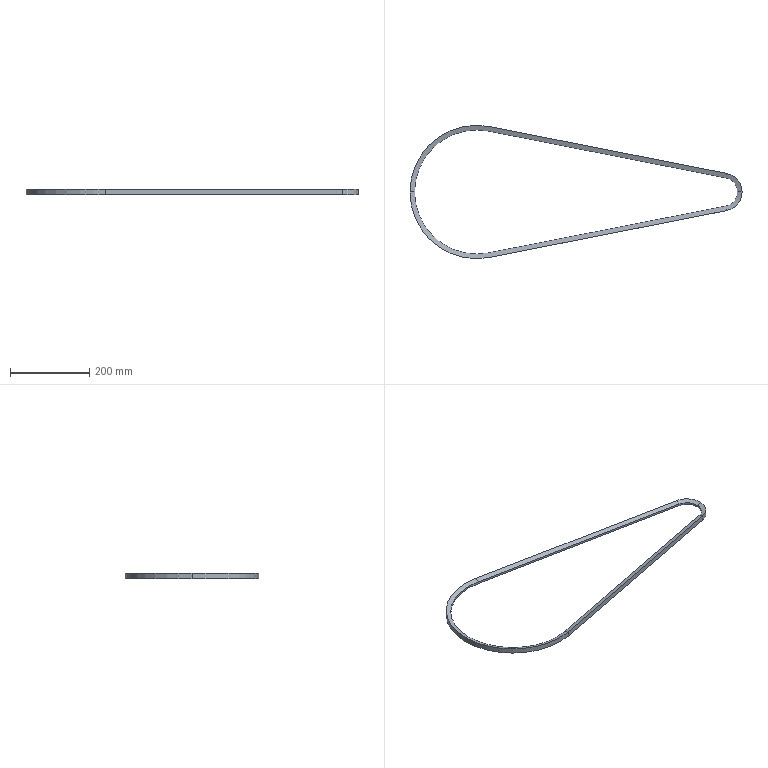Part | SolidWorks | features Sweep 1 | 1 solid | 21 faces | box 835.6 x 335.6 x 13 mm | volume 197670 mm3 | plane 8 | cone 7 | cylinder 6 | commonest cylinder face diameters 312.6 x2 335.6 x2 72.6 x1 95.6 x1
STEP:
#1=CARTESIAN_POINT('',(627.026,35.614,5.));
#2=VERTEX_POINT('',#1);
#3=CARTESIAN_POINT('',(656.3,0.,5.));
#4=VERTEX_POINT('',#3);
#5=CARTESIAN_POINT('',(620.,0.,5.));
#6=DIRECTION('',(0.,0.,-1.));
#7=DIRECTION('',(0.1935,0.9811,0.));
#8=AXIS2_PLACEMENT_3D('',#5,#6,#7);
#9=CIRCLE('',#8,36.3);
#10=EDGE_CURVE('',#2,#4,#9,.T.);
#11=ORIENTED_EDGE('',*,*,#10,.T.);
#12=CARTESIAN_POINT('',(667.8,0.,9.));
#13=VERTEX_POINT('',#12);
#14=CARTESIAN_POINT('',(667.8,0.,9.));
#15=DIRECTION('',(0.9445,0.,0.3285));
#16=VECTOR('',#15,1000.);
#17=LINE('',#14,#16);
#18=EDGE_CURVE('',#4,#13,#17,.T.);
#19=ORIENTED_EDGE('',*,*,#18,.T.);
#20=CARTESIAN_POINT('',(629.252,46.896,9.));
#21=VERTEX_POINT('',#20);
#22=CARTESIAN_POINT('',(620.,0.,9.));
#23=DIRECTION('',(0.,0.,-1.));
#24=DIRECTION('',(0.1935,0.9811,0.));
#25=AXIS2_PLACEMENT_3D('',#22,#23,#24);
#26=CIRCLE('',#25,47.8);
#27=EDGE_CURVE('',#21,#13,#26,.T.);
#28=ORIENTED_EDGE('',*,*,#27,.F.);
#29=CARTESIAN_POINT('',(627.026,35.614,5.));
#30=DIRECTION('',(-0.1828,-0.9266,-0.3285));
#31=VECTOR('',#30,1000.);
#32=LINE('',#29,#31);
#33=EDGE_CURVE('',#21,#2,#32,.T.);
#34=ORIENTED_EDGE('',*,*,#33,.T.);
#35=EDGE_LOOP('',(#11,#19,#28,#34));
#36=FACE_OUTER_BOUND('',#35,.T.);
#37=CARTESIAN_POINT('',(620.,0.,9.));
#38=DIRECTION('',(0.,0.,1.));
#39=DIRECTION('',(1.,0.,0.));
#40=AXIS2_PLACEMENT_3D('',#37,#38,#39);
#41=CONICAL_SURFACE('',#40,47.8,1.236);
#42=ADVANCED_FACE('',(#36),#41,.F.);
#43=CARTESIAN_POINT('',(30.252,-153.344,5.));
#44=VERTEX_POINT('',#43);
#45=CARTESIAN_POINT('',(-156.3,0.,5.));
#46=VERTEX_POINT('',#45);
#47=CARTESIAN_POINT('',(0.,0.,5.));
#48=DIRECTION('',(0.,0.,-1.));
#49=DIRECTION('',(0.1935,-0.9811,0.));
#50=AXIS2_PLACEMENT_3D('',#47,#48,#49);
#51=CIRCLE('',#50,156.3);
#52=EDGE_CURVE('',#44,#46,#51,.T.);
#53=ORIENTED_EDGE('',*,*,#52,.F.);
#54=CARTESIAN_POINT('',(30.252,-153.344,0.));
#55=VERTEX_POINT('',#54);
#56=CARTESIAN_POINT('',(30.252,-153.344,0.));
#57=DIRECTION('',(0.,0.,-1.));
#58=VECTOR('',#57,1000.);
#59=LINE('',#56,#58);
#60=EDGE_CURVE('',#44,#55,#59,.T.);
#61=ORIENTED_EDGE('',*,*,#60,.T.);
#62=CARTESIAN_POINT('',(-156.3,0.,0.));
#63=VERTEX_POINT('',#62);
#64=CARTESIAN_POINT('',(0.,0.,0.));
#65=DIRECTION('',(0.,0.,-1.));
#66=DIRECTION('',(0.1935,-0.9811,0.));
#67=AXIS2_PLACEMENT_3D('',#64,#65,#66);
#68=CIRCLE('',#67,156.3);
#69=EDGE_CURVE('',#55,#63,#68,.T.);
#70=ORIENTED_EDGE('',*,*,#69,.T.);
#71=CARTESIAN_POINT('',(-156.3,0.,0.));
#72=DIRECTION('',(0.,0.,-1.));
#73=VECTOR('',#72,1000.);
#74=LINE('',#71,#73);
#75=EDGE_CURVE('',#46,#63,#74,.T.);
#76=ORIENTED_EDGE('',*,*,#75,.F.);
#77=EDGE_LOOP('',(#53,#61,#70,#76));
#78=FACE_OUTER_BOUND('',#77,.T.);
#79=CARTESIAN_POINT('',(0.,0.,0.));
#80=DIRECTION('',(0.,0.,-1.));
#81=DIRECTION('',(-1.,0.,0.));
#82=AXIS2_PLACEMENT_3D('',#79,#80,#81);
#83=CYLINDRICAL_SURFACE('',#82,156.3);
#84=ADVANCED_FACE('',(#78),#83,.F.);
#85=CARTESIAN_POINT('',(32.477,-164.627,9.));
#86=VERTEX_POINT('',#85);
#87=CARTESIAN_POINT('',(-167.8,0.,9.));
#88=VERTEX_POINT('',#87);
#89=CARTESIAN_POINT('',(0.,0.,9.));
#90=DIRECTION('',(0.,0.,-1.));
#91=DIRECTION('',(0.1935,-0.9811,0.));
#92=AXIS2_PLACEMENT_3D('',#89,#90,#91);
#93=CIRCLE('',#92,167.8);
#94=EDGE_CURVE('',#86,#88,#93,.T.);
#95=ORIENTED_EDGE('',*,*,#94,.F.);
#96=CARTESIAN_POINT('',(30.252,-153.344,5.));
#97=DIRECTION('',(-0.1828,0.9266,-0.3285));
#98=VECTOR('',#97,1000.);
#99=LINE('',#96,#98);
#100=EDGE_CURVE('',#86,#44,#99,.T.);
#101=ORIENTED_EDGE('',*,*,#100,.T.);
#102=ORIENTED_EDGE('',*,*,#52,.T.);
#103=CARTESIAN_POINT('',(-156.3,0.,5.));
#104=DIRECTION('',(0.9445,0.,-0.3285));
#105=VECTOR('',#104,1000.);
#106=LINE('',#103,#105);
#107=EDGE_CURVE('',#88,#46,#106,.T.);
#108=ORIENTED_EDGE('',*,*,#107,.F.);
#109=EDGE_LOOP('',(#95,#101,#102,#108));
#110=FACE_OUTER_BOUND('',#109,.T.);
#111=CARTESIAN_POINT('',(0.,0.,9.));
#112=DIRECTION('',(0.,0.,1.));
#113=DIRECTION('',(1.,0.,0.));
#114=AXIS2_PLACEMENT_3D('',#111,#112,#113);
#115=CONICAL_SURFACE('',#114,167.8,1.236);
#116=ADVANCED_FACE('',(#110),#115,.F.);
#117=CARTESIAN_POINT('',(32.477,-164.627,-4.));
#118=VERTEX_POINT('',#117);
#119=CARTESIAN_POINT('',(-167.8,0.,-4.));
#120=VERTEX_POINT('',#119);
#121=CARTESIAN_POINT('',(0.,0.,-4.));
#122=DIRECTION('',(0.,0.,-1.));
#123=DIRECTION('',(0.1935,-0.9811,0.));
#124=AXIS2_PLACEMENT_3D('',#121,#122,#123);
#125=CIRCLE('',#124,167.8);
#126=EDGE_CURVE('',#118,#120,#125,.T.);
#127=ORIENTED_EDGE('',*,*,#126,.F.);
#128=CARTESIAN_POINT('',(32.477,-164.627,-4.));
#129=DIRECTION('',(0.,0.,1.));
#130=VECTOR('',#129,1000.);
#131=LINE('',#128,#130);
#132=EDGE_CURVE('',#118,#86,#131,.T.);
#133=ORIENTED_EDGE('',*,*,#132,.T.);
#134=ORIENTED_EDGE('',*,*,#94,.T.);
#135=CARTESIAN_POINT('',(-167.8,0.,-4.));
#136=DIRECTION('',(0.,0.,1.));
#137=VECTOR('',#136,1000.);
#138=LINE('',#135,#137);
#139=EDGE_CURVE('',#120,#88,#138,.T.);
#140=ORIENTED_EDGE('',*,*,#139,.F.);
#141=EDGE_LOOP('',(#127,#133,#134,#140));
#142=FACE_OUTER_BOUND('',#141,.T.);
#143=CARTESIAN_POINT('',(0.,0.,0.));
#144=DIRECTION('',(0.,0.,-1.));
#145=DIRECTION('',(-1.,0.,0.));
#146=AXIS2_PLACEMENT_3D('',#143,#144,#145);
#147=CYLINDRICAL_SURFACE('',#146,167.8);
#148=ADVANCED_FACE('',(#142),#147,.T.);
#149=ORIENTED_EDGE('',*,*,#60,.F.);
#150=CARTESIAN_POINT('',(627.026,-35.614,5.));
#151=VERTEX_POINT('',#150);
#152=CARTESIAN_POINT('',(627.026,-35.614,5.));
#153=DIRECTION('',(-0.9811,-0.1935,0.));
#154=VECTOR('',#153,1000.);
#155=LINE('',#152,#154);
#156=EDGE_CURVE('',#151,#44,#155,.T.);
#157=ORIENTED_EDGE('',*,*,#156,.F.);
#158=CARTESIAN_POINT('',(627.026,-35.614,0.));
#159=VERTEX_POINT('',#158);
#160=CARTESIAN_POINT('',(627.026,-35.614,0.));
#161=DIRECTION('',(0.,0.,-1.));
#162=VECTOR('',#161,1000.);
#163=LINE('',#160,#162);
#164=EDGE_CURVE('',#151,#159,#163,.T.);
#165=ORIENTED_EDGE('',*,*,#164,.T.);
#166=CARTESIAN_POINT('',(627.026,-35.614,0.));
#167=DIRECTION('',(-0.9811,-0.1935,0.));
#168=VECTOR('',#167,1000.);
#169=LINE('',#166,#168);
#170=EDGE_CURVE('',#159,#55,#169,.T.);
#171=ORIENTED_EDGE('',*,*,#170,.T.);
#172=EDGE_LOOP('',(#149,#157,#165,#171));
#173=FACE_OUTER_BOUND('',#172,.T.);
#174=CARTESIAN_POINT('',(627.026,-35.614,0.));
#175=DIRECTION('',(-0.1935,0.9811,0.));
#176=DIRECTION('',(-0.9811,-0.1935,0.));
#177=AXIS2_PLACEMENT_3D('',#174,#175,#176);
#178=PLANE('',#177);
#179=ADVANCED_FACE('',(#173),#178,.T.);
#180=ORIENTED_EDGE('',*,*,#156,.T.);
#181=ORIENTED_EDGE('',*,*,#100,.F.);
#182=CARTESIAN_POINT('',(629.252,-46.896,9.));
#183=VERTEX_POINT('',#182);
#184=CARTESIAN_POINT('',(629.252,-46.896,9.));
#185=DIRECTION('',(-0.9811,-0.1935,0.));
#186=VECTOR('',#185,1000.);
#187=LINE('',#184,#186);
#188=EDGE_CURVE('',#183,#86,#187,.T.);
#189=ORIENTED_EDGE('',*,*,#188,.F.);
#190=CARTESIAN_POINT('',(627.026,-35.614,5.));
#191=DIRECTION('',(-0.1828,0.9266,-0.3285));
#192=VECTOR('',#191,1000.);
#193=LINE('',#190,#192);
#194=EDGE_CURVE('',#183,#151,#193,.T.);
#195=ORIENTED_EDGE('',*,*,#194,.T.);
#196=EDGE_LOOP('',(#180,#181,#189,#195));
#197=FACE_OUTER_BOUND('',#196,.T.);
#198=CARTESIAN_POINT('',(627.026,-35.614,5.));
#199=DIRECTION('',(-0.06358,0.3223,0.9445));
#200=DIRECTION('',(0.,-0.9464,0.323));
#201=AXIS2_PLACEMENT_3D('',#198,#199,#200);
#202=PLANE('',#201);
#203=ADVANCED_FACE('',(#197),#202,.T.);
#204=ORIENTED_EDGE('',*,*,#188,.T.);
#205=ORIENTED_EDGE('',*,*,#132,.F.);
#206=CARTESIAN_POINT('',(629.252,-46.896,-4.));
#207=VERTEX_POINT('',#206);
#208=CARTESIAN_POINT('',(629.252,-46.896,-4.));
#209=DIRECTION('',(-0.9811,-0.1935,0.));
#210=VECTOR('',#209,1000.);
#211=LINE('',#208,#210);
#212=EDGE_CURVE('',#207,#118,#211,.T.);
#213=ORIENTED_EDGE('',*,*,#212,.F.);
#214=CARTESIAN_POINT('',(629.252,-46.896,-4.));
#215=DIRECTION('',(0.,0.,1.));
#216=VECTOR('',#215,1000.);
#217=LINE('',#214,#216);
#218=EDGE_CURVE('',#207,#183,#217,.T.);
#219=ORIENTED_EDGE('',*,*,#218,.T.);
#220=EDGE_LOOP('',(#204,#205,#213,#219));
#221=FACE_OUTER_BOUND('',#220,.T.);
#222=CARTESIAN_POINT('',(629.252,-46.896,-4.));
#223=DIRECTION('',(0.1935,-0.9811,0.));
#224=DIRECTION('',(0.9811,0.1935,0.));
#225=AXIS2_PLACEMENT_3D('',#222,#223,#224);
#226=PLANE('',#225);
#227=ADVANCED_FACE('',(#221),#226,.T.);
#228=ORIENTED_EDGE('',*,*,#212,.T.);
#229=CARTESIAN_POINT('',(32.477,-164.627,-4.));
#230=DIRECTION('',(0.1828,-0.9266,-0.3285));
#231=VECTOR('',#230,1000.);
#232=LINE('',#229,#231);
#233=EDGE_CURVE('',#55,#118,#232,.T.);
#234=ORIENTED_EDGE('',*,*,#233,.F.);
#235=ORIENTED_EDGE('',*,*,#170,.F.);
#236=CARTESIAN_POINT('',(629.252,-46.896,-4.));
#237=DIRECTION('',(0.1828,-0.9266,-0.3285));
#238=VECTOR('',#237,1000.);
#239=LINE('',#236,#238);
#240=EDGE_CURVE('',#159,#207,#239,.T.);
#241=ORIENTED_EDGE('',*,*,#240,.T.);
#242=EDGE_LOOP('',(#228,#234,#235,#241));
#243=FACE_OUTER_BOUND('',#242,.T.);
#244=CARTESIAN_POINT('',(629.252,-46.896,-4.));
#245=DIRECTION('',(-0.06358,0.3223,-0.9445));
#246=DIRECTION('',(0.,0.9464,0.323));
#247=AXIS2_PLACEMENT_3D('',#244,#245,#246);
#248=PLANE('',#247);
#249=ADVANCED_FACE('',(#243),#248,.T.);
#250=ORIENTED_EDGE('',*,*,#164,.F.);
#251=CARTESIAN_POINT('',(620.,0.,5.));
#252=DIRECTION('',(0.,0.,-1.));
#253=DIRECTION('',(0.1935,0.9811,0.));
#254=AXIS2_PLACEMENT_3D('',#251,#252,#253);
#255=CIRCLE('',#254,36.3);
#256=EDGE_CURVE('',#4,#151,#255,.T.);
#257=ORIENTED_EDGE('',*,*,#256,.F.);
#258=ORIENTED_EDGE('',*,*,#10,.F.);
#259=CARTESIAN_POINT('',(627.026,35.614,0.));
#260=VERTEX_POINT('',#259);
#261=CARTESIAN_POINT('',(627.026,35.614,0.));
#262=DIRECTION('',(0.,0.,-1.));
#263=VECTOR('',#262,1000.);
#264=LINE('',#261,#263);
#265=EDGE_CURVE('',#2,#260,#264,.T.);
#266=ORIENTED_EDGE('',*,*,#265,.T.);
#267=CARTESIAN_POINT('',(620.,0.,0.));
#268=DIRECTION('',(0.,0.,-1.));
#269=DIRECTION('',(0.1935,0.9811,0.));
#270=AXIS2_PLACEMENT_3D('',#267,#268,#269);
#271=CIRCLE('',#270,36.3);
#272=EDGE_CURVE('',#260,#159,#271,.T.);
#273=ORIENTED_EDGE('',*,*,#272,.T.);
#274=EDGE_LOOP('',(#250,#257,#258,#266,#273));
#275=FACE_OUTER_BOUND('',#274,.T.);
#276=CARTESIAN_POINT('',(620.,0.,0.));
#277=DIRECTION('',(0.,0.,-1.));
#278=DIRECTION('',(-1.,0.,0.));
#279=AXIS2_PLACEMENT_3D('',#276,#277,#278);
#280=CYLINDRICAL_SURFACE('',#279,36.3);
#281=ADVANCED_FACE('',(#275),#280,.F.);
#282=ORIENTED_EDGE('',*,*,#18,.F.);
#283=ORIENTED_EDGE('',*,*,#256,.T.);
#284=ORIENTED_EDGE('',*,*,#194,.F.);
#285=CARTESIAN_POINT('',(620.,0.,9.));
#286=DIRECTION('',(0.,0.,-1.));
#287=DIRECTION('',(0.1935,0.9811,0.));
#288=AXIS2_PLACEMENT_3D('',#285,#286,#287);
#289=CIRCLE('',#288,47.8);
#290=EDGE_CURVE('',#13,#183,#289,.T.);
#291=ORIENTED_EDGE('',*,*,#290,.F.);
#292=EDGE_LOOP('',(#282,#283,#284,#291));
#293=FACE_OUTER_BOUND('',#292,.T.);
#294=CARTESIAN_POINT('',(620.,0.,9.));
#295=DIRECTION('',(0.,0.,1.));
#296=DIRECTION('',(1.,0.,0.));
#297=AXIS2_PLACEMENT_3D('',#294,#295,#296);
#298=CONICAL_SURFACE('',#297,47.8,1.236);
#299=ADVANCED_FACE('',(#293),#298,.F.);
#300=ORIENTED_EDGE('',*,*,#27,.T.);
#301=ORIENTED_EDGE('',*,*,#290,.T.);
#302=ORIENTED_EDGE('',*,*,#218,.F.);
#303=CARTESIAN_POINT('',(629.252,46.896,-4.));
#304=VERTEX_POINT('',#303);
#305=CARTESIAN_POINT('',(620.,0.,-4.));
#306=DIRECTION('',(0.,0.,-1.));
#307=DIRECTION('',(0.1935,0.9811,0.));
#308=AXIS2_PLACEMENT_3D('',#305,#306,#307);
#309=CIRCLE('',#308,47.8);
#310=EDGE_CURVE('',#304,#207,#309,.T.);
#311=ORIENTED_EDGE('',*,*,#310,.F.);
#312=CARTESIAN_POINT('',(629.252,46.896,-4.));
#313=DIRECTION('',(0.,0.,1.));
#314=VECTOR('',#313,1000.);
#315=LINE('',#312,#314);
#316=EDGE_CURVE('',#304,#21,#315,.T.);
#317=ORIENTED_EDGE('',*,*,#316,.T.);
#318=EDGE_LOOP('',(#300,#301,#302,#311,#317));
#319=FACE_OUTER_BOUND('',#318,.T.);
#320=CARTESIAN_POINT('',(620.,0.,0.));
#321=DIRECTION('',(0.,0.,-1.));
#322=DIRECTION('',(-1.,0.,0.));
#323=AXIS2_PLACEMENT_3D('',#320,#321,#322);
#324=CYLINDRICAL_SURFACE('',#323,47.8);
#325=ADVANCED_FACE('',(#319),#324,.T.);
#326=ORIENTED_EDGE('',*,*,#310,.T.);
#327=ORIENTED_EDGE('',*,*,#240,.F.);
#328=ORIENTED_EDGE('',*,*,#272,.F.);
#329=CARTESIAN_POINT('',(629.252,46.896,-4.));
#330=DIRECTION('',(0.1828,0.9266,-0.3285));
#331=VECTOR('',#330,1000.);
#332=LINE('',#329,#331);
#333=EDGE_CURVE('',#260,#304,#332,.T.);
#334=ORIENTED_EDGE('',*,*,#333,.T.);
#335=EDGE_LOOP('',(#326,#327,#328,#334));
#336=FACE_OUTER_BOUND('',#335,.T.);
#337=CARTESIAN_POINT('',(620.,0.,0.));
#338=DIRECTION('',(0.,0.,-1.));
#339=DIRECTION('',(-1.,0.,0.));
#340=AXIS2_PLACEMENT_3D('',#337,#338,#339);
#341=CONICAL_SURFACE('',#340,36.3,1.236);
#342=ADVANCED_FACE('',(#336),#341,.F.);
#343=ORIENTED_EDGE('',*,*,#265,.F.);
#344=CARTESIAN_POINT('',(30.252,153.344,5.));
#345=VERTEX_POINT('',#344);
#346=CARTESIAN_POINT('',(30.252,153.344,5.));
#347=DIRECTION('',(0.9811,-0.1935,0.));
#348=VECTOR('',#347,1000.);
#349=LINE('',#346,#348);
#350=EDGE_CURVE('',#345,#2,#349,.T.);
#351=ORIENTED_EDGE('',*,*,#350,.F.);
#352=CARTESIAN_POINT('',(30.252,153.344,0.));
#353=VERTEX_POINT('',#352);
#354=CARTESIAN_POINT('',(30.252,153.344,0.));
#355=DIRECTION('',(0.,0.,-1.));
#356=VECTOR('',#355,1000.);
#357=LINE('',#354,#356);
#358=EDGE_CURVE('',#345,#353,#357,.T.);
#359=ORIENTED_EDGE('',*,*,#358,.T.);
#360=CARTESIAN_POINT('',(30.252,153.344,0.));
#361=DIRECTION('',(0.9811,-0.1935,0.));
#362=VECTOR('',#361,1000.);
#363=LINE('',#360,#362);
#364=EDGE_CURVE('',#353,#260,#363,.T.);
#365=ORIENTED_EDGE('',*,*,#364,.T.);
#366=EDGE_LOOP('',(#343,#351,#359,#365));
#367=FACE_OUTER_BOUND('',#366,.T.);
#368=CARTESIAN_POINT('',(30.252,153.344,0.));
#369=DIRECTION('',(-0.1935,-0.9811,0.));
#370=DIRECTION('',(0.9811,-0.1935,0.));
#371=AXIS2_PLACEMENT_3D('',#368,#369,#370);
#372=PLANE('',#371);
#373=ADVANCED_FACE('',(#367),#372,.T.);
#374=ORIENTED_EDGE('',*,*,#350,.T.);
#375=ORIENTED_EDGE('',*,*,#33,.F.);
#376=CARTESIAN_POINT('',(32.477,164.627,9.));
#377=VERTEX_POINT('',#376);
#378=CARTESIAN_POINT('',(32.477,164.627,9.));
#379=DIRECTION('',(0.9811,-0.1935,0.));
#380=VECTOR('',#379,1000.);
#381=LINE('',#378,#380);
#382=EDGE_CURVE('',#377,#21,#381,.T.);
#383=ORIENTED_EDGE('',*,*,#382,.F.);
#384=CARTESIAN_POINT('',(30.252,153.344,5.));
#385=DIRECTION('',(-0.1828,-0.9266,-0.3285));
#386=VECTOR('',#385,1000.);
#387=LINE('',#384,#386);
#388=EDGE_CURVE('',#377,#345,#387,.T.);
#389=ORIENTED_EDGE('',*,*,#388,.T.);
#390=EDGE_LOOP('',(#374,#375,#383,#389));
#391=FACE_OUTER_BOUND('',#390,.T.);
#392=CARTESIAN_POINT('',(30.252,153.344,5.));
#393=DIRECTION('',(-0.06358,-0.3223,0.9445));
#394=DIRECTION('',(0.,-0.9464,-0.323));
#395=AXIS2_PLACEMENT_3D('',#392,#393,#394);
#396=PLANE('',#395);
#397=ADVANCED_FACE('',(#391),#396,.T.);
#398=ORIENTED_EDGE('',*,*,#382,.T.);
#399=ORIENTED_EDGE('',*,*,#316,.F.);
#400=CARTESIAN_POINT('',(32.477,164.627,-4.));
#401=VERTEX_POINT('',#400);
#402=CARTESIAN_POINT('',(32.477,164.627,-4.));
#403=DIRECTION('',(0.9811,-0.1935,0.));
#404=VECTOR('',#403,1000.);
#405=LINE('',#402,#404);
#406=EDGE_CURVE('',#401,#304,#405,.T.);
#407=ORIENTED_EDGE('',*,*,#406,.F.);
#408=CARTESIAN_POINT('',(32.477,164.627,-4.));
#409=DIRECTION('',(0.,0.,1.));
#410=VECTOR('',#409,1000.);
#411=LINE('',#408,#410);
#412=EDGE_CURVE('',#401,#377,#411,.T.);
#413=ORIENTED_EDGE('',*,*,#412,.T.);
#414=EDGE_LOOP('',(#398,#399,#407,#413));
#415=FACE_OUTER_BOUND('',#414,.T.);
#416=CARTESIAN_POINT('',(32.477,164.627,-4.));
#417=DIRECTION('',(0.1935,0.9811,0.));
#418=DIRECTION('',(-0.9811,0.1935,0.));
#419=AXIS2_PLACEMENT_3D('',#416,#417,#418);
#420=PLANE('',#419);
#421=ADVANCED_FACE('',(#415),#420,.T.);
#422=ORIENTED_EDGE('',*,*,#406,.T.);
#423=ORIENTED_EDGE('',*,*,#333,.F.);
#424=ORIENTED_EDGE('',*,*,#364,.F.);
#425=CARTESIAN_POINT('',(32.477,164.627,-4.));
#426=DIRECTION('',(0.1828,0.9266,-0.3285));
#427=VECTOR('',#426,1000.);
#428=LINE('',#425,#427);
#429=EDGE_CURVE('',#353,#401,#428,.T.);
#430=ORIENTED_EDGE('',*,*,#429,.T.);
#431=EDGE_LOOP('',(#422,#423,#424,#430));
#432=FACE_OUTER_BOUND('',#431,.T.);
#433=CARTESIAN_POINT('',(32.477,164.627,-4.));
#434=DIRECTION('',(-0.06358,-0.3223,-0.9445));
#435=DIRECTION('',(0.,0.9464,-0.323));
#436=AXIS2_PLACEMENT_3D('',#433,#434,#435);
#437=PLANE('',#436);
#438=ADVANCED_FACE('',(#432),#437,.T.);
#439=ORIENTED_EDGE('',*,*,#358,.F.);
#440=CARTESIAN_POINT('',(0.,0.,5.));
#441=DIRECTION('',(0.,0.,-1.));
#442=DIRECTION('',(-1.,0.,0.));
#443=AXIS2_PLACEMENT_3D('',#440,#441,#442);
#444=CIRCLE('',#443,156.3);
#445=EDGE_CURVE('',#46,#345,#444,.T.);
#446=ORIENTED_EDGE('',*,*,#445,.F.);
#447=ORIENTED_EDGE('',*,*,#75,.T.);
#448=CARTESIAN_POINT('',(0.,0.,0.));
#449=DIRECTION('',(0.,0.,-1.));
#450=DIRECTION('',(-1.,0.,0.));
#451=AXIS2_PLACEMENT_3D('',#448,#449,#450);
#452=CIRCLE('',#451,156.3);
#453=EDGE_CURVE('',#63,#353,#452,.T.);
#454=ORIENTED_EDGE('',*,*,#453,.T.);
#455=EDGE_LOOP('',(#439,#446,#447,#454));
#456=FACE_OUTER_BOUND('',#455,.T.);
#457=CARTESIAN_POINT('',(0.,0.,0.));
#458=DIRECTION('',(0.,0.,-1.));
#459=DIRECTION('',(-1.,0.,0.));
#460=AXIS2_PLACEMENT_3D('',#457,#458,#459);
#461=CYLINDRICAL_SURFACE('',#460,156.3);
#462=ADVANCED_FACE('',(#456),#461,.F.);
#463=ORIENTED_EDGE('',*,*,#445,.T.);
#464=ORIENTED_EDGE('',*,*,#388,.F.);
#465=CARTESIAN_POINT('',(0.,0.,9.));
#466=DIRECTION('',(0.,0.,-1.));
#467=DIRECTION('',(-1.,0.,0.));
#468=AXIS2_PLACEMENT_3D('',#465,#466,#467);
#469=CIRCLE('',#468,167.8);
#470=EDGE_CURVE('',#88,#377,#469,.T.);
#471=ORIENTED_EDGE('',*,*,#470,.F.);
#472=ORIENTED_EDGE('',*,*,#107,.T.);
#473=EDGE_LOOP('',(#463,#464,#471,#472));
#474=FACE_OUTER_BOUND('',#473,.T.);
#475=CARTESIAN_POINT('',(0.,0.,9.));
#476=DIRECTION('',(0.,0.,1.));
#477=DIRECTION('',(1.,0.,0.));
#478=AXIS2_PLACEMENT_3D('',#475,#476,#477);
#479=CONICAL_SURFACE('',#478,167.8,1.236);
#480=ADVANCED_FACE('',(#474),#479,.F.);
#481=ORIENTED_EDGE('',*,*,#470,.T.);
#482=ORIENTED_EDGE('',*,*,#412,.F.);
#483=CARTESIAN_POINT('',(0.,0.,-4.));
#484=DIRECTION('',(0.,0.,-1.));
#485=DIRECTION('',(-1.,0.,0.));
#486=AXIS2_PLACEMENT_3D('',#483,#484,#485);
#487=CIRCLE('',#486,167.8);
#488=EDGE_CURVE('',#120,#401,#487,.T.);
#489=ORIENTED_EDGE('',*,*,#488,.F.);
#490=ORIENTED_EDGE('',*,*,#139,.T.);
#491=EDGE_LOOP('',(#481,#482,#489,#490));
#492=FACE_OUTER_BOUND('',#491,.T.);
#493=CARTESIAN_POINT('',(0.,0.,0.));
#494=DIRECTION('',(0.,0.,-1.));
#495=DIRECTION('',(-1.,0.,0.));
#496=AXIS2_PLACEMENT_3D('',#493,#494,#495);
#497=CYLINDRICAL_SURFACE('',#496,167.8);
#498=ADVANCED_FACE('',(#492),#497,.T.);
#499=ORIENTED_EDGE('',*,*,#488,.T.);
#500=ORIENTED_EDGE('',*,*,#429,.F.);
#501=ORIENTED_EDGE('',*,*,#453,.F.);
#502=CARTESIAN_POINT('',(-167.8,0.,-4.));
#503=DIRECTION('',(-0.9445,0.,-0.3285));
#504=VECTOR('',#503,1000.);
#505=LINE('',#502,#504);
#506=EDGE_CURVE('',#63,#120,#505,.T.);
#507=ORIENTED_EDGE('',*,*,#506,.T.);
#508=EDGE_LOOP('',(#499,#500,#501,#507));
#509=FACE_OUTER_BOUND('',#508,.T.);
#510=CARTESIAN_POINT('',(0.,0.,0.));
#511=DIRECTION('',(0.,0.,-1.));
#512=DIRECTION('',(-1.,0.,0.));
#513=AXIS2_PLACEMENT_3D('',#510,#511,#512);
#514=CONICAL_SURFACE('',#513,156.3,1.236);
#515=ADVANCED_FACE('',(#509),#514,.F.);
#516=ORIENTED_EDGE('',*,*,#233,.T.);
#517=ORIENTED_EDGE('',*,*,#126,.T.);
#518=ORIENTED_EDGE('',*,*,#506,.F.);
#519=ORIENTED_EDGE('',*,*,#69,.F.);
#520=EDGE_LOOP('',(#516,#517,#518,#519));
#521=FACE_OUTER_BOUND('',#520,.T.);
#522=CARTESIAN_POINT('',(0.,0.,0.));
#523=DIRECTION('',(0.,0.,-1.));
#524=DIRECTION('',(-1.,0.,0.));
#525=AXIS2_PLACEMENT_3D('',#522,#523,#524);
#526=CONICAL_SURFACE('',#525,156.3,1.236);
#527=ADVANCED_FACE('',(#521),#526,.F.);
#528=CLOSED_SHELL('',(#42,#84,#116,#148,#179,#203,#227,#249,#281,#299,#325,#342,#373,#397,#421,#438,#462,#480,#498,#515,#527));
#529=MANIFOLD_SOLID_BREP('',#528);
#530=CARTESIAN_POINT('',(0.,0.,0.));
#531=DIRECTION('',(0.,0.,1.));
#532=DIRECTION('',(1.,0.,0.));
#533=AXIS2_PLACEMENT_3D('',#530,#531,#532);
#534=(LENGTH_UNIT()NAMED_UNIT(*)SI_UNIT(.MILLI.,.METRE.));
#535=UNCERTAINTY_MEASURE_WITH_UNIT(LENGTH_MEASURE(0.00001),#534,'','');
#536=(NAMED_UNIT(*)PLANE_ANGLE_UNIT()SI_UNIT($,.RADIAN.));
#537=(NAMED_UNIT(*)SI_UNIT($,.STERADIAN.)SOLID_ANGLE_UNIT());
#538=(GEOMETRIC_REPRESENTATION_CONTEXT(3)GLOBAL_UNCERTAINTY_ASSIGNED_CONTEXT((#535))GLOBAL_UNIT_ASSIGNED_CONTEXT((#534,#536,#537))REPRESENTATION_CONTEXT('',''));
#539=ADVANCED_BREP_SHAPE_REPRESENTATION('',(#529,#533),#538);